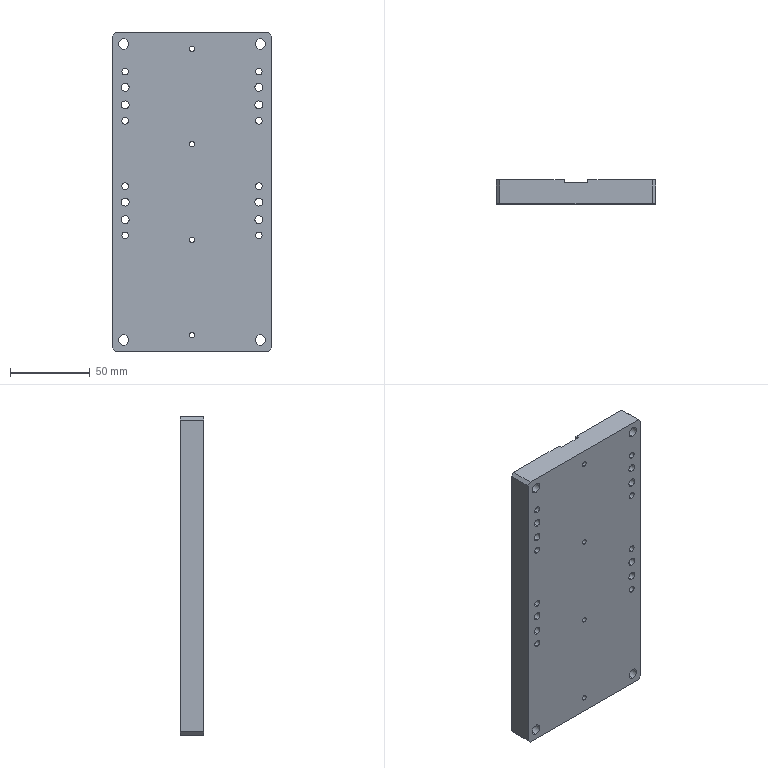Part | STEP file | 11-FG-E01111 | 1 solid | 74 faces | box 100 x 15 x 200 mm | volume 285807 mm3 | cylinder 56 | plane 18 | commonest cylinder face diameters 4.2 x16 5 x16 3.3 x8 6.6 x8 11 x8